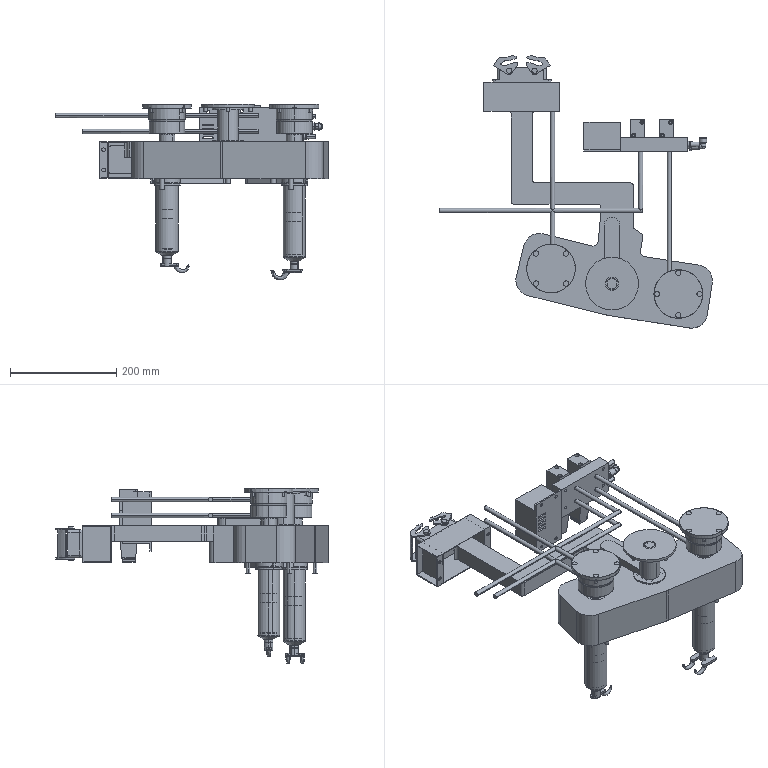Part | STEP file | COMPOUND | 37 solids | 1859 faces | box 514.266 x 513.429 x 330.33 mm | volume 7966584 mm3 | cylinder 734 | plane 592 | cone 349 | spline 81 | torus 56 | sphere 37 | other 10 | commonest cylinder face diameters 8 x72 10 x67 3 x46 4 x45 6 x36 7 x32